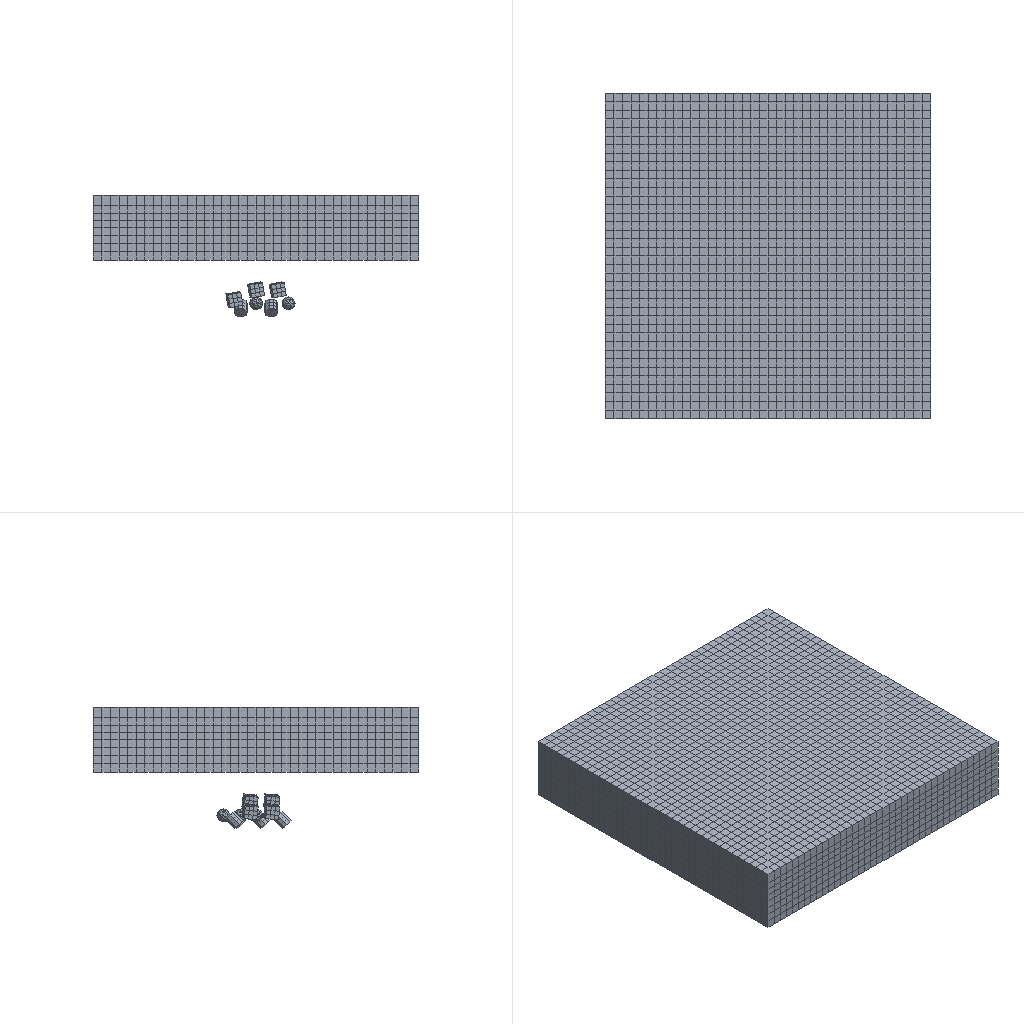Simulation study | abaqus
Set-up summary:
category,name,step,type,value,unit,region
solver,abaqus
solver,version,,,Abaqus/Standard 2020
units,not stated in the deck,,not stated
analysis,deck,,transient,transient
load_step,Step-1,Step-1,transient
load_step,requested,,,1
mesh,nodes,,,19847
mesh,elements,,,15155
element_type,C3D8R,,solid,11870
element_type,C3D10M,,solid,3285
load,load commands in deck,,count,1
bc,support commands in deck,,count,1
material,NIANTU,,in results
material,SHATU,,in results
material,SHI,,in results
material,YUNI,,in results
check,setup vs results,,match,"per instance, exact: element labels, types and connectivity; labels of the nodes the elements use; coordinates of those nodes at SINGLE_PRECISION in 15 of 16 instance(s)"
Abaqus input file, long lists of numbers shortened:
*Heading
** Job name: Job-1 Model name: Model-1
** Generated by: Abaqus/CAE 2020
*Preprint, echo=NO, model=NO, history=NO, contact=NO
**
** PARTS
**
*Part, name=base
*Node
      1,           0.,           0.,          1.5
      2,           0.,         -15.,          1.5
** (13687 more lines like these left out)
*Element, type=C3D8R
   1,  246,  925, 6845,  777,    1,   17,  629,   94
   2,  925,  926, 6846, 6845,   17,   18,  630,  629
** (11550 more lines like these left out)
*Nset, nset=Set-1
    3,    4,    6,    7,   13,   14,   15,   16,   56,   57,   58,   59,   60,   61,   62,   63
   64,   65,   66,   67,   68,   69,   70,   71,   72,   73,   74,   75,   76,   77,   78,   79
** (189 more lines like these left out)
*Elset, elset=Set-1, generate
 10109,  11552,      1
*Nset, nset=Set-2
    1,    2,    3,    4,    5,    6,    7,    8,   17,   18,   19,   20,   21,   22,   23,   24
   25,   26,   27,   28,   29,   30,   31,   32,   33,   34,   35,   36,   37,   38,   39,   40
** (379 more lines like these left out)
*Elset, elset=Set-2, generate
    1,  4332,     1
*Nset, nset=Set-3
     1,     2,     5,     8,     9,    10,    11,    12,    17,    18,    19,    20,    21,    22,    23,    24
    25,    26,    27,    28,    29,    30,    31,    32,    33,    34,    35,    36,    37,    38,    39,    40
** (474 more lines like these left out)
*Elset, elset=Set-3, generate
  4333,  10108,      1
** Section: niantu
*Solid Section, elset=Set-2, material=niantu
,
** Section: shatu
*Solid Section, elset=Set-3, material=shatu
,
** Section: yuni
*Solid Section, elset=Set-1, material=yuni
,
*End Part
**
*Part, name=fang
*Node
      1,           0., -0.6,  0.6
      2,           0., -0.4,  0.6
** (62 more lines like these left out)
*Element, type=C3D8R
 1, 17, 18, 22, 21,  1,  2,  6,  5
 2, 18, 19, 23, 22,  2,  3,  7,  6
** (25 more lines like these left out)
*Nset, nset=Set-1, generate
  1,  64,   1
*Elset, elset=Set-1, generate
  1,  27,   1
** Section: shi
*Solid Section, elset=Set-1, material=shi
,
*End Part
**
*Part, name=fangkuai
*Node
      1,  0.2427,           0.,  0.1763
      2, 0.09271,           0.,  0.2853
** (74 more lines like these left out)
*Element, type=C3D8R
 1,  6,  7,  8, 19, 25, 26, 27, 38
 2, 11, 14, 12, 19, 30, 33, 31, 38
** (37 more lines like these left out)
*Nset, nset=Set-1, generate
  1,  76,   1
*Elset, elset=Set-1, generate
  1,  39,   1
** Section: shi
*Solid Section, elset=Set-1, material=shi
,
*End Part
**
*Part, name=sphere
*Node
      1,  0.1148,  0.2772,           0.
      2,  0.2121,  0.2121,           0.
** (1092 more lines like these left out)
*Element, type=C3D10M
  1,  101,  102,  103,  104,  173,  172,  171,  175,  174,  176
  2,  105,  106,  102,  107,  179,  178,  177,  181,  180,  182
** (655 more lines like these left out)
*Nset, nset=Set-1, generate
    1,  1094,     1
*Elset, elset=Set-1, generate
   1,  657,    1
** Section: shi
*Solid Section, elset=Set-1, material=shi
,
*End Part
**
**
** ASSEMBLY
**
*Assembly, name=Assembly
**
*Instance, name=base-1, part=base
*End Instance
**
*Instance, name=sphere-1, part=sphere
         7.5,         -7.5,          -2.
*End Instance
**
*Instance, name=fangkuai-1, part=fangkuai
         8.2,         -7.5,          -2.
         8.2,         -7.5,          -2., 9.2,         -7.5,          -2., 45.
*End Instance
**
*Instance, name=fang-1, part=fang
6.209, -6.949, -2.154
6.209, -6.949, -2.154, 6.542, -7.616, -1.487, 15.
*End Instance
**
*Instance, name=sphere-1-lin-1-2, part=sphere
         7.5,         -6.8,          -2.
*End Instance
**
*Instance, name=sphere-1-lin-2-1, part=sphere
          9.,         -7.5,          -2.
*End Instance
**
*Instance, name=sphere-1-lin-2-2, part=sphere
          9.,         -6.8,          -2.
*End Instance
**
*Instance, name=fangkuai-1-lin-1-2, part=fangkuai
         8.2,         -6.4,          -2.
         8.2,         -6.4,          -2., 9.2,         -6.4,          -2., 45.
*End Instance
**
*Instance, name=fangkuai-1-lin-1-2-1, part=fangkuai
         8.2,         -8.5,          -2.
         8.2,         -8.5,          -2., 9.2,         -8.5,          -2., 45.
*End Instance
**
*Instance, name=fang-1-lin-1-2, part=fang
6.209, -7.949, -2.154
6.209, -7.949, -2.154, 6.542, -8.616, -1.487, 15.
*End Instance
**
*Instance, name=fang-1-lin-2-1, part=fang
7.209, -6.949, -1.704
7.209, -6.949, -1.704, 7.542, -7.616, -1.037, 15.
*End Instance
**
*Instance, name=fang-1-lin-2-2, part=fang
7.209, -7.949, -1.704
7.209, -7.949, -1.704, 7.542, -8.616, -1.037, 15.
*End Instance
**
*Instance, name=fang-1-lin-3-1, part=fang
8.209, -6.949, -1.704
8.209, -6.949, -1.704, 8.542, -7.616, -1.037, 15.
*End Instance
**
*Instance, name=fang-1-lin-3-2, part=fang
8.209, -7.949, -1.704
8.209, -7.949, -1.704, 8.542, -8.616, -1.037, 15.
*End Instance
**
*Instance, name=sphere-1-lin-1-2-lin-1-2, part=sphere
         7.5,          -6.,          -2.
*End Instance
**
*Instance, name=fangkuai-1-lin-1-2-lin-2-1, part=fangkuai
         6.8,         -6.3,          -2.
         6.8,         -6.3,          -2., 7.8,         -6.3,          -2., 45.
*End Instance
**
*Nset, nset=Set-1, instance=base-1
   13,   14,   15,   16,  481,  482,  483,  484,  485,  486,  487,  488,  489,  490,  491,  492
  493,  494,  495,  496,  497,  498,  499,  500,  501,  502,  503,  504,  505,  506,  507,  508
** (94 more lines like these left out)
*Elset, elset=Set-1, instance=base-1, generate
 10109,  11552,      1
*Nset, nset=Set-2, instance=sphere-1, generate
    1,  1094,     1
*Nset, nset=Set-2, instance=fangkuai-1, generate
  1,  76,   1
*Nset, nset=Set-2, instance=fang-1, generate
  1,  64,   1
*Nset, nset=Set-2, instance=fangkuai-1-lin-1-2, generate
  1,  76,   1
*Nset, nset=Set-2, instance=fangkuai-1-lin-1-2-lin-2-1, generate
  1,  76,   1
*Nset, nset=Set-2, instance=fang-1-lin-2-2, generate
  1,  64,   1
*Nset, nset=Set-2, instance=sphere-1-lin-2-1, generate
    1,  1094,     1
*Nset, nset=Set-2, instance=fang-1-lin-1-2, generate
  1,  64,   1
*Nset, nset=Set-2, instance=fang-1-lin-3-2, generate
  1,  64,   1
*Nset, nset=Set-2, instance=sphere-1-lin-1-2, generate
    1,  1094,     1
*Nset, nset=Set-2, instance=fangkuai-1-lin-1-2-1, generate
  1,  76,   1
*Nset, nset=Set-2, instance=fang-1-lin-3-1, generate
  1,  64,   1
*Nset, nset=Set-2, instance=sphere-1-lin-2-2, generate
    1,  1094,     1
*Nset, nset=Set-2, instance=fang-1-lin-2-1, generate
  1,  64,   1
*Nset, nset=Set-2, instance=sphere-1-lin-1-2-lin-1-2, generate
    1,  1094,     1
*Elset, elset=Set-2, instance=sphere-1, generate
   1,  657,    1
*Elset, elset=Set-2, instance=fangkuai-1, generate
  1,  39,   1
*Elset, elset=Set-2, instance=fang-1, generate
  1,  27,   1
*Elset, elset=Set-2, instance=fangkuai-1-lin-1-2, generate
  1,  39,   1
*Elset, elset=Set-2, instance=fangkuai-1-lin-1-2-lin-2-1, generate
  1,  39,   1
*Elset, elset=Set-2, instance=fang-1-lin-2-2, generate
  1,  27,   1
*Elset, elset=Set-2, instance=sphere-1-lin-2-1, generate
   1,  657,    1
*Elset, elset=Set-2, instance=fang-1-lin-1-2, generate
  1,  27,   1
*Elset, elset=Set-2, instance=fang-1-lin-3-2, generate
  1,  27,   1
*Elset, elset=Set-2, instance=sphere-1-lin-1-2, generate
   1,  657,    1
*Elset, elset=Set-2, instance=fangkuai-1-lin-1-2-1, generate
  1,  39,   1
*Elset, elset=Set-2, instance=fang-1-lin-3-1, generate
  1,  27,   1
*Elset, elset=Set-2, instance=sphere-1-lin-2-2, generate
   1,  657,    1
*Elset, elset=Set-2, instance=fang-1-lin-2-1, generate
  1,  27,   1
*Elset, elset=Set-2, instance=sphere-1-lin-1-2-lin-1-2, generate
   1,  657,    1
*Elset, elset=__Int-1_gcs0_17_S3, internal, instance=sphere-1
  37,  61,  70,  92, 110, 121, 137, 145, 146, 173, 197, 218, 224, 238, 277, 286
 298, 300, 327, 346, 399, 405, 411, 412, 414, 415, 421, 422, 425, 428, 434, 437
** (9 more lines like these left out)
*Elset, elset=__Int-1_gcs0_17_S4, internal, instance=sphere-1
  53,  84, 112, 166, 184, 251, 264, 265, 320, 624, 655
*Elset, elset=__Int-1_gcs0_17_S1, internal, instance=sphere-1
  67, 293, 381, 419
*Elset, elset=__Int-1_gcs0_17_S2, internal, instance=sphere-1
 220, 350, 409, 427, 447, 451, 588, 650
*Surface, type=ELEMENT, name=_Int-1_gcs0_17, internal
__Int-1_gcs0_17_S3, S3
__Int-1_gcs0_17_S4, S4
__Int-1_gcs0_17_S2, S2
__Int-1_gcs0_17_S1, S1
*Elset, elset=__Int-1_gcs0_18_S3, internal, instance=fangkuai-1
  1,  8, 14, 21, 27, 34
*Elset, elset=__Int-1_gcs0_18_S4, internal, instance=fangkuai-1
  1,  3,  4, 13, 14, 16, 17, 26, 27, 29, 30, 39
*Elset, elset=__Int-1_gcs0_18_S5, internal, instance=fangkuai-1
  5,  6, 11, 18, 19, 24, 31, 32, 37
*Elset, elset=__Int-1_gcs0_18_S6, internal, instance=fangkuai-1, generate
 10,  36,  13
*Surface, type=ELEMENT, name=_Int-1_gcs0_18, internal
__Int-1_gcs0_18_S3, S3
__Int-1_gcs0_18_S4, S4
__Int-1_gcs0_18_S6, S6
__Int-1_gcs0_18_S5, S5
*Elset, elset=__Int-1_gcs0_27_S3, internal, instance=sphere-1-lin-1-2
  37,  61,  70,  92, 110, 121, 137, 145, 146, 173, 197, 218, 224, 238, 277, 286
 298, 300, 327, 346, 399, 405, 411, 412, 414, 415, 421, 422, 425, 428, 434, 437
** (9 more lines like these left out)
*Elset, elset=__Int-1_gcs0_27_S4, internal, instance=sphere-1-lin-1-2
  53,  84, 112, 166, 184, 251, 264, 265, 320, 624, 655
*Elset, elset=__Int-1_gcs0_27_S1, internal, instance=sphere-1-lin-1-2
  67, 293, 381, 419
*Elset, elset=__Int-1_gcs0_27_S2, internal, instance=sphere-1-lin-1-2
 220, 350, 409, 427, 447, 451, 588, 650
*Surface, type=ELEMENT, name=_Int-1_gcs0_27, internal
__Int-1_gcs0_27_S3, S3
__Int-1_gcs0_27_S4, S4
__Int-1_gcs0_27_S2, S2
__Int-1_gcs0_27_S1, S1
*Elset, elset=__Int-1_gcs0_28_S3, internal, instance=sphere-1-lin-2-1
  37,  61,  70,  92, 110, 121, 137, 145, 146, 173, 197, 218, 224, 238, 277, 286
 298, 300, 327, 346, 399, 405, 411, 412, 414, 415, 421, 422, 425, 428, 434, 437
** (9 more lines like these left out)
*Elset, elset=__Int-1_gcs0_28_S4, internal, instance=sphere-1-lin-2-1
  53,  84, 112, 166, 184, 251, 264, 265, 320, 624, 655
*Elset, elset=__Int-1_gcs0_28_S1, internal, instance=sphere-1-lin-2-1
  67, 293, 381, 419
*Elset, elset=__Int-1_gcs0_28_S2, internal, instance=sphere-1-lin-2-1
 220, 350, 409, 427, 447, 451, 588, 650
*Surface, type=ELEMENT, name=_Int-1_gcs0_28, internal
__Int-1_gcs0_28_S3, S3
__Int-1_gcs0_28_S4, S4
__Int-1_gcs0_28_S2, S2
__Int-1_gcs0_28_S1, S1
*Elset, elset=__Int-1_gcs0_29_S3, internal, instance=sphere-1-lin-2-2
  37,  61,  70,  92, 110, 121, 137, 145, 146, 173, 197, 218, 224, 238, 277, 286
 298, 300, 327, 346, 399, 405, 411, 412, 414, 415, 421, 422, 425, 428, 434, 437
** (9 more lines like these left out)
*Elset, elset=__Int-1_gcs0_29_S4, internal, instance=sphere-1-lin-2-2
  53,  84, 112, 166, 184, 251, 264, 265, 320, 624, 655
*Elset, elset=__Int-1_gcs0_29_S1, internal, instance=sphere-1-lin-2-2
  67, 293, 381, 419
*Elset, elset=__Int-1_gcs0_29_S2, internal, instance=sphere-1-lin-2-2
 220, 350, 409, 427, 447, 451, 588, 650
*Surface, type=ELEMENT, name=_Int-1_gcs0_29, internal
__Int-1_gcs0_29_S3, S3
__Int-1_gcs0_29_S4, S4
__Int-1_gcs0_29_S2, S2
__Int-1_gcs0_29_S1, S1
*Elset, elset=__Int-1_gcs0_30_S3, internal, instance=fangkuai-1-lin-1-2
  1,  8, 14, 21, 27, 34
*Elset, elset=__Int-1_gcs0_30_S4, internal, instance=fangkuai-1-lin-1-2
  1,  3,  4, 13, 14, 16, 17, 26, 27, 29, 30, 39
*Elset, elset=__Int-1_gcs0_30_S5, internal, instance=fangkuai-1-lin-1-2
  5,  6, 11, 18, 19, 24, 31, 32, 37
*Elset, elset=__Int-1_gcs0_30_S6, internal, instance=fangkuai-1-lin-1-2, generate
 10,  36,  13
*Surface, type=ELEMENT, name=_Int-1_gcs0_30, internal
__Int-1_gcs0_30_S3, S3
__Int-1_gcs0_30_S4, S4
__Int-1_gcs0_30_S6, S6
__Int-1_gcs0_30_S5, S5
*Elset, elset=__Int-1_gcs0_33_S3, internal, instance=fangkuai-1-lin-1-2-1
  1,  8, 14, 21, 27, 34
*Elset, elset=__Int-1_gcs0_33_S4, internal, instance=fangkuai-1-lin-1-2-1
  1,  3,  4, 13, 14, 16, 17, 26, 27, 29, 30, 39
*Elset, elset=__Int-1_gcs0_33_S5, internal, instance=fangkuai-1-lin-1-2-1
  5,  6, 11, 18, 19, 24, 31, 32, 37
*Elset, elset=__Int-1_gcs0_33_S6, internal, instance=fangkuai-1-lin-1-2-1, generate
 10,  36,  13
*Surface, type=ELEMENT, name=_Int-1_gcs0_33, internal
__Int-1_gcs0_33_S3, S3
__Int-1_gcs0_33_S4, S4
__Int-1_gcs0_33_S6, S6
__Int-1_gcs0_33_S5, S5
*Elset, elset=__Int-1_gcs0_66_S3, internal, instance=sphere-1-lin-1-2-lin-1-2
  37,  61,  70,  92, 110, 121, 137, 145, 146, 173, 197, 218, 224, 238, 277, 286
 298, 300, 327, 346, 399, 405, 411, 412, 414, 415, 421, 422, 425, 428, 434, 437
** (9 more lines like these left out)
*Elset, elset=__Int-1_gcs0_66_S4, internal, instance=sphere-1-lin-1-2-lin-1-2
  53,  84, 112, 166, 184, 251, 264, 265, 320, 624, 655
*Elset, elset=__Int-1_gcs0_66_S1, internal, instance=sphere-1-lin-1-2-lin-1-2
  67, 293, 381, 419
*Elset, elset=__Int-1_gcs0_66_S2, internal, instance=sphere-1-lin-1-2-lin-1-2
 220, 350, 409, 427, 447, 451, 588, 650
*Surface, type=ELEMENT, name=_Int-1_gcs0_66, internal
__Int-1_gcs0_66_S3, S3
__Int-1_gcs0_66_S4, S4
__Int-1_gcs0_66_S2, S2
__Int-1_gcs0_66_S1, S1
*Elset, elset=__Int-1_gcs0_67_S3, internal, instance=fangkuai-1-lin-1-2-lin-2-1
  1,  8, 14, 21, 27, 34
*Elset, elset=__Int-1_gcs0_67_S4, internal, instance=fangkuai-1-lin-1-2-lin-2-1
  1,  3,  4, 13, 14, 16, 17, 26, 27, 29, 30, 39
*Elset, elset=__Int-1_gcs0_67_S5, internal, instance=fangkuai-1-lin-1-2-lin-2-1
  5,  6, 11, 18, 19, 24, 31, 32, 37
*Elset, elset=__Int-1_gcs0_67_S6, internal, instance=fangkuai-1-lin-1-2-lin-2-1, generate
 10,  36,  13
*Surface, type=ELEMENT, name=_Int-1_gcs0_67, internal
__Int-1_gcs0_67_S3, S3
__Int-1_gcs0_67_S4, S4
__Int-1_gcs0_67_S6, S6
__Int-1_gcs0_67_S5, S5
*End Assembly
**
** MATERIALS
**
*Material, name=niantu
*Density
1700.,
*Elastic
 6e+08, 0.35
*Material, name=shatu
*Density
2300.,
*Elastic
 2e+09, 0.36
*Material, name=shi
*Density
2850.,
*Elastic
 2e+10, 0.22
*Material, name=yuni
*Density
1400.,
*Elastic
 6e+09, 0.35
**
** INTERACTION PROPERTIES
**
*Surface Interaction, name=IntProp-1
1.,
*Friction, slip tolerance=0.005
 0.2,
*Surface Behavior, pressure-overclosure=HARD
**
** INTERACTIONS
**
** Interaction: Int-1
*Contact
*Contact Inclusions, ALL EXTERIOR
*Contact Property Assignment
 ,  , IntProp-1
*Surface Property Assignment, property=GEOMETRIC CORRECTION
_Int-1_gcs0_17, Spherical, 7.5, -7.5, -2.
_Int-1_gcs0_18, Circumferential, 8.2, -7.712, -2.212,  8.2, -8.419, -2.919
_Int-1_gcs0_27, Spherical, 7.5, -6.8, -2.
_Int-1_gcs0_28, Spherical, 9., -7.5, -2.
_Int-1_gcs0_29, Spherical, 9., -6.8, -2.
_Int-1_gcs0_30, Circumferential, 8.2, -6.612, -2.212,  8.2, -7.319, -2.919
_Int-1_gcs0_33, Circumferential, 8.2, -8.712, -2.212,  8.2, -9.419, -2.919
_Int-1_gcs0_66, Spherical, 7.5, -6., -2.
_Int-1_gcs0_67, Circumferential, 6.8, -6.512, -2.212,  6.8, -7.219, -2.919
** ----------------------------------------------------------------
**
** STEP: Step-1
**
*Step, name=Step-1, nlgeom=YES, inc=1000
*Dynamic
0.01,1.,1e-05
**
** BOUNDARY CONDITIONS
**
** Name: BC-1 Type: 对称/反对称/完全固定
*Boundary
Set-1, ENCASTRE
**
** LOADS
**
** Name: Load-1   Type: Gravity
*Dload
Set-2, GRAV, 9.8, 0., 0., 1.
**
** OUTPUT REQUESTS
**
*Restart, write, number interval=1, time marks=NO
**
** FIELD OUTPUT: F-Output-1
**
*Output, field, variable=PRESELECT, number interval=50, time marks=NO
**
** HISTORY OUTPUT: H-Output-1
**
*Output, history, variable=PRESELECT, number interval=200, time marks=NO
*End Step
Results summary:
result,step,,completed,increments=177 time=1.0/1.0
result,analysis,,,transient
result,last_loadstep,,,1
result,primary field,,,U
result,reaction total,,FX,-34664.559,model units
result,reaction total,,FY,-20246.128,model units
result,reaction total,,FZ,-102434.681,model units